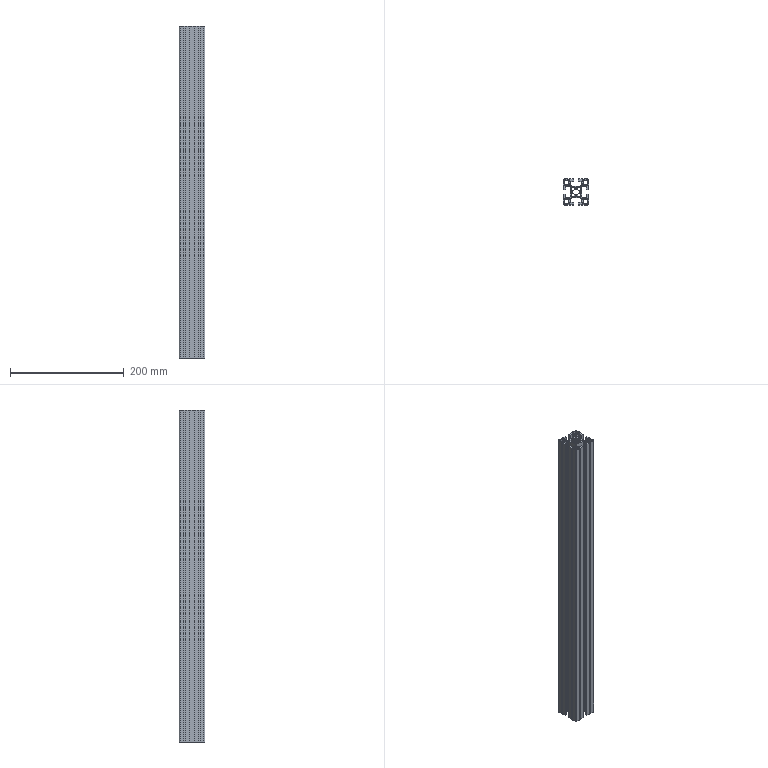Part | STEP file | 4545 profile NG mount | 1 solid | 262 faces | box 45 x 45 x 585 mm | volume 405901 mm3 | plane 186 | cylinder 76 | commonest cylinder face diameters 2 x44 8 x20 12 x8 4 x4